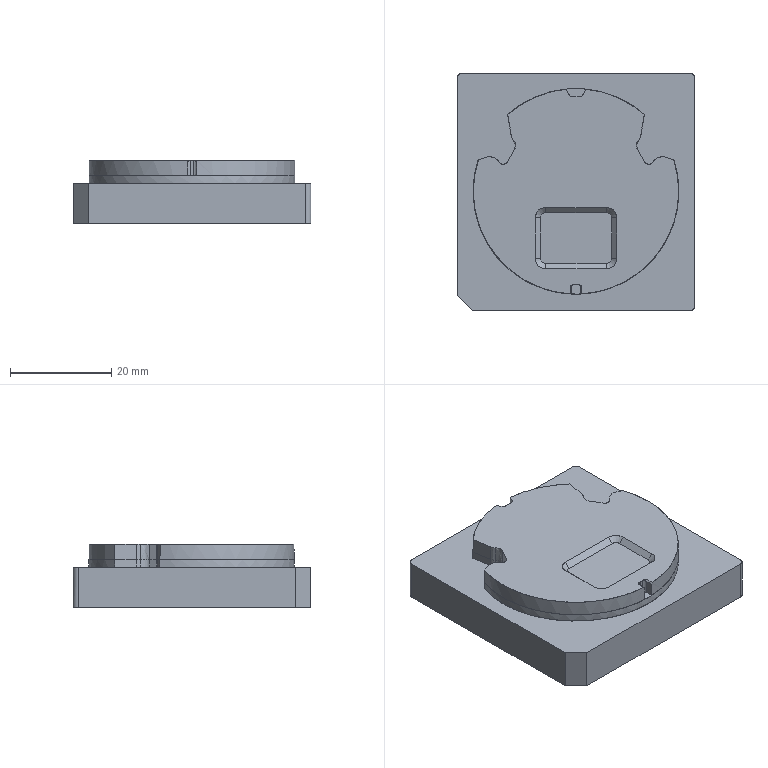NC program | PowerMill | posted with a generic post | part box 47 x 47 x 12.511 mm
Lines 3814 to 4800 of 232111:
N3911 M6
N3912 S18000 M03
N3913 G00 G90 X0.0 Y0.0
N3914 G43 Z9.8015 H15
N3915
N3916 G05 P10000 R4
N3917 X15.7379 Y13.9176
N3918 Z0.8545
N3919 G01 Z-0.3455 F3000.0
N3920 X15.7225 Y13.9292 F5000.0
N3921 G03 X15.48 Y13.8941 I-0.1037 J-0.1388
N3922 G01 X14.5606 Y12.664
N3923 X14.1805 Y10.5533
N3924 X14.048 Y10.1312
N3925 X13.8339 Y9.7091
N3926 X13.4893 Y9.2284
N3927 X13.4614 Y9.1489
N3928 X13.4808 Y9.0669
N3929 X14.3834 Y7.477
N3930 G03 X14.6063 Y7.433 I0.1304 J0.074
N3931 G01 X15.1968 Y7.8958
N3932 X15.6189 Y8.1199
N3933 X16.0411 Y8.2805
N3934 X16.4632 Y8.3842
N3935 X16.8682 Y8.4427
N3936 X17.3146
N3937 X17.7296 Y8.4111
N3938 X18.5739 Y8.1829
N3939 X19.8403 Y7.72
N3940 X20.0941 Y7.5984
N3941 X20.2624 Y7.4819
N3942 X20.5487 Y7.1763
N3943 X20.6845 Y6.9495
N3944 X20.9948 Y5.9099
N3945 X21.2205 Y5.0656
N3946 X21.5288 Y3.5136
N3947 X21.6562 Y2.5328
N3948 X21.7637 Y1.2664
N3949 X21.786 Y0.4221
N3950 X21.7476 Y-1.2664
N3951 X21.5716 Y-2.9549
N3952 X21.3505 Y-4.2213
N3953 X20.9434 Y-5.9099
N3954 X20.5366 Y-7.1763
N3955 X20.0398 Y-8.4427
N3956 X19.4181 Y-9.776
N3957 X18.7603 Y-10.9755
N3958 X17.951 Y-12.2419
N3959 X17.0083 Y-13.5083
N3960 X15.9126 Y-14.7747
N3961 X14.7747 Y-15.9019
N3962 X13.5083 Y-16.9858
N3963 X12.664 Y-17.6049
N3964 X11.8804 Y-18.1517
N3965 X10.5533 Y-18.9524
N3966 X9.2869 Y-19.5988
N3967 X7.7239 Y-20.2624
N3968 X6.4951 Y-20.6845
N3969 X5.0656 Y-21.0791
N3970 X3.7992 Y-21.3429
N3971 X2.5376 Y-21.5288
N3972 X1.2664 Y-21.6389
N3973 X0.8443 Y-21.6396
N3974 X0.4341 Y-21.5288
N3975 X0.0829 Y-21.2972
N3976 X0.0001 Y-21.2725
N3977 X-0.0827 Y-21.2975
N3978 X-0.4221 Y-21.5232
N3979 X-0.8443 Y-21.6396
N3980 X-1.2664 Y-21.6389
N3981 X-2.5375 Y-21.5288
N3982 X-3.7992 Y-21.3429
N3983 X-5.0656 Y-21.0791
N3984 X-6.4951 Y-20.6845
N3985 X-7.7269 Y-20.2624
N3986 X-8.7488 Y-19.8403
N3987 X-10.1312 Y-19.179
N3988 X-11.2043 Y-18.5739
N3989 X-12.2419 Y-17.9036
N3990 X-13.5083 Y-16.9805
N3991 X-14.6241 Y-16.0411
N3992 X-15.5066 Y-15.1968
N3993 X-15.9121 Y-14.7747
N3994 X-16.8853 Y-13.6622
N3995 X-17.9488 Y-12.2419
N3996 X-18.7581 Y-10.9755
N3997 X-19.4181 Y-9.776
N3998 X-20.0398 Y-8.4427
N3999 X-20.5365 Y-7.1763
N4000 X-20.9434 Y-5.9099
N4001 X-21.2664 Y-4.6435
N4002 X-21.5288 Y-3.2569
N4003 X-21.7173 Y-1.6885
N4004 X-21.7801 Y-0.4221
N4005 X-21.7637 Y1.2664
N4006 X-21.6562 Y2.5328
N4007 X-21.5288 Y3.5149
N4008 X-21.4005 Y4.2213
N4009 X-21.121 Y5.4877
N4010 X-20.6845 Y6.9495
N4011 X-20.5503 Y7.1763
N4012 X-20.2624 Y7.4819
N4013 X-20.0957 Y7.5984
N4014 X-19.8403 Y7.72
N4015 X-18.5739 Y8.1829
N4016 X-17.7296 Y8.4111
N4017 X-17.3075 Y8.4433
N4018 X-16.8853 Y8.4434
N4019 X-16.4632 Y8.3842
N4020 X-16.0411 Y8.2805
N4021 X-15.6189 Y8.1199
N4022 X-15.1968 Y7.8958
N4023 X-14.7747 Y7.5787
N4024 X-14.6138 Y7.4355
N4025 G03 X-14.3778 Y7.4835 I0.0999 J0.1129
N4026 G01 X-13.576 Y8.8648
N4027 X-13.4828 Y9.0677
N4028 X-13.4697 Y9.1433
N4029 X-13.4958 Y9.2156
N4030 X-13.837 Y9.7091
N4031 X-14.048 Y10.1312
N4032 X-14.1814 Y10.5533
N4033 X-14.3525 Y11.428
N4034 X-15.0027 Y15.1968
N4035 X-14.9617 Y15.6189
N4036 X-14.7907 Y16.0411
N4037 X-14.3525 Y16.5091
N4038 X-13.5083 Y17.2179
N4039 X-12.2308 Y18.1517
N4040 X-11.3976 Y18.6865
N4041 X-10.1135 Y19.4181
N4042 X-8.8648 Y20.0225
N4043 X-7.5984 Y20.5388
N4044 X-6.332 Y20.966
N4045 X-5.0656 Y21.3114
N4046 X-3.3771 Y21.6465
N4047 X-2.1107 Y21.809
N4048 X-1.6885 Y21.8011
N4049 X-1.2664 Y21.6731
N4050 X-1.0252 Y21.5288
N4051 X-0.8443 Y21.373
N4052 X-0.6349 Y21.1067
N4053 X-0.3437 Y20.503
N4054 X-0.2885 Y20.4413
N4055 X-0.2089 Y20.4182
N4056 X0.2081 Y20.4173
N4057 X0.2877 Y20.4399
N4058 X0.3431 Y20.5012
N4059 X0.6402 Y21.1067
N4060 X0.8443 Y21.373
N4061 X1.0221 Y21.5288
N4062 X1.2664 Y21.6731
N4063 X1.6885 Y21.8011
N4064 X2.1107 Y21.809
N4065 X3.3771 Y21.6465
N4066 X4.6435 Y21.406
N4067 X6.332 Y20.966
N4068 X7.5984 Y20.5388
N4069 X8.8648 Y20.0225
N4070 X10.1312 Y19.4083
N4071 X10.8809 Y18.996
N4072 X12.2419 Y18.1446
N4073 X13.3961 Y17.3075
N4074 X14.4068 Y16.4632
N4075 X14.7747 Y16.0676
N4076 X14.9617 Y15.6189
N4077 X15.0027 Y15.1968
N4078 X14.9408 Y14.7747
N4079 X14.5606 Y12.664
N4080 X15.7379 Y13.9207 Z-0.4819
N4081 X15.7225 Y13.9322
N4082 G03 X15.4801 Y13.8967 I-0.1035 J-0.139
N4083 G01 X14.5623 Y12.6637
N4084 X14.3734 Y11.6083
N4085 X14.1826 Y10.5533
N4086 X14.0498 Y10.1312
N4087 X13.8389 Y9.7091
N4088 X13.4878 Y9.2236
N4089 X13.48 Y9.2088
N4090 X13.4631 Y9.1479
N4091 X13.4733 Y9.0856
N4092 X13.4807 Y9.0669
N4093 X14.3774 Y7.4874
N4094 X14.385 Y7.4754
N4095 X14.3937 Y7.4641
N4096 G03 X14.6056 Y7.4341 I0.1201 J0.0845
N4097 G01 X15.1968 Y7.8973
N4098 X15.6189 Y8.1199
N4099 X16.0411 Y8.2822
N4100 X16.4632 Y8.3842
N4101 X16.8455 Y8.4427
N4102 X17.3146
N4103 X17.7296 Y8.412
N4104 X18.5739 Y8.1841
N4105 X19.8403 Y7.7215
N4106 X20.0981 Y7.5984
N4107 X20.2624 Y7.4845
N4108 X20.5543 Y7.1763
N4109 X20.6845 Y6.9524
N4110 X20.7592 Y6.7541
N4111 X20.946 Y6.0734
N4112 X20.9948 Y5.9099
N4113 X21.145 Y5.3481
N4114 X21.2224 Y5.0656
N4115 X21.5288 Y3.5216
N4116 X21.6562 Y2.5328
N4117 X21.7637 Y1.2664
N4118 X21.7879 Y0.4221
N4119 X21.7489 Y-1.2664
N4120 X21.5732 Y-2.9549
N4121 X21.4247 Y-3.8001
N4122 X21.2667 Y-4.6435
N4123 X20.9434 Y-5.9099
N4124 X20.5366 Y-7.1763
N4125 X20.0398 Y-8.4427
N4126 X19.4181 Y-9.776
N4127 X18.7617 Y-10.9755
N4128 X17.9511 Y-12.2419
N4129 X17.9311 Y-12.2686
N4130 X17.0083 Y-13.5082
N4131 X16.9663 Y-13.5567
N4132 X16.8853 Y-13.6649
N4133 X16.4632 Y-14.1597
N4134 X16.183 Y-14.4628
N4135 X15.9126 Y-14.7746
N4136 X15.7049 Y-14.9811
N4137 X15.5067 Y-15.1968
N4138 X14.8424 Y-15.8348
N4139 X14.7746 Y-15.9019
N4140 X14.755 Y-15.9187
N4141 X14.6276 Y-16.0411
N4142 X13.5083 Y-16.9858
N4143 X12.7021 Y-17.5773
N4144 X11.8837 Y-18.1517
N4145 X10.5533 Y-18.9538
N4146 X9.2869 Y-19.5989
N4147 X9.2363 Y-19.6203
N4148 X7.7239 Y-20.2624
N4149 X7.6482 Y-20.2883
N4150 X7.5984 Y-20.3093
N4151 X7.3606 Y-20.3872
N4152 X6.4951 Y-20.6845
N4153 X6.2004 Y-20.7664
N4154 X5.9099 Y-20.8621
N4155 X5.0656 Y-21.0791
N4156 X4.2213 Y-21.263
N4157 X4.0093 Y-21.2978
N4158 X3.7992 Y-21.3428
N4159 X2.6329 Y-21.5147
N4160 X2.5439 Y-21.5288
N4161 X1.2664 Y-21.6392
N4162 X0.8443 Y-21.6495
N4163 X0.4221 Y-21.5713
N4164 X0.3134 Y-21.5288
N4165 X0.0739 Y-21.3845
N4166 X-0.0005 Y-21.363
N4167 X-0.0756 Y-21.3814
N4168 X-0.4221 Y-21.5713
N4169 X-0.8443 Y-21.6495
N4170 X-1.2664 Y-21.6392
N4171 X-2.5419 Y-21.5288
N4172 X-3.3771 Y-21.4061
N4173 X-3.4088 Y-21.4003
N4174 X-3.7992 Y-21.3428
N4175 X-4.433 Y-21.2139
N4176 X-5.0656 Y-21.0791
N4177 X-5.4862 Y-20.9648
N4178 X-5.9099 Y-20.8621
N4179 X-6.2003 Y-20.7661
N4180 X-6.4951 Y-20.6845
N4181 X-7.6618 Y-20.2847
N4182 X-7.7372 Y-20.2595
N4183 X-7.8101 Y-20.228
N4184 X-8.7488 Y-19.8402
N4185 X-9.0152 Y-19.7136
N4186 X-9.2869 Y-19.5986
N4187 X-9.8824 Y-19.3
N4188 X-10.475 Y-18.996
N4189 X-10.837 Y-18.7802
N4190 X-11.2043 Y-18.5738
N4191 X-11.5416 Y-18.3569
N4192 X-11.8861 Y-18.1517
N4193 X-12.5052 Y-17.7296
N4194 X-13.5083 Y-16.983
N4195 X-14.6273 Y-16.0411
N4196 X-14.7473 Y-15.9231
N4197 X-15.5066 Y-15.1968
N4198 X-15.8535 Y-14.8357
N4199 X-15.9155 Y-14.7747
N4200 X-16.8853 Y-13.6649
N4201 X-17.9508 Y-12.2419
N4202 X-18.76 Y-10.9755
N4203 X-18.9495 Y-10.641
N4204 X-19.1291 Y-10.3012
N4205 X-19.4181 Y-9.776
N4206 X-19.5335 Y-9.5287
N4207 X-19.6602 Y-9.2869
N4208 X-19.9644 Y-8.6022
N4209 X-20.2624 Y-7.9147
N4210 X-20.3927 Y-7.543
N4211 X-20.5365 Y-7.1763
N4212 X-20.7435 Y-6.5442
N4213 X-20.9433 Y-5.9099
N4214 X-21.2004 Y-4.9021
N4215 X-21.2697 Y-4.6435
N4216 X-21.5288 Y-3.2633
N4217 X-21.7179 Y-1.6885
N4218 X-21.721 Y-1.6137
N4219 X-21.78 Y-0.4221
N4220 X-21.7785 Y-0.211
N4221 X-21.7877 Y0.0
N4222 X-21.7637 Y1.2664
N4223 X-21.6562 Y2.5328
N4224 X-21.6555 Y2.5376
N4225 X-21.5288 Y3.5149
N4226 X-21.4005 Y4.2213
N4227 X-21.1231 Y5.478
N4228 X-21.121 Y5.4877
N4229 X-20.7601 Y6.7541
N4230 X-20.6845 Y6.9524
N4231 X-20.553 Y7.1763
N4232 X-20.2624 Y7.4845
N4233 X-20.1003 Y7.5984
N4234 X-19.8403 Y7.7215
N4235 X-18.5739 Y8.1841
N4236 X-17.7296 Y8.412
N4237 X-17.3075 Y8.4438
N4238 X-17.0998 Y8.4433
N4239 X-16.8853 Y8.4434
N4240 X-16.8786 Y8.4429
N4241 X-16.8719 Y8.4427
N4242 X-16.8464
N4243 X-16.4632 Y8.3842
N4244 X-16.0411 Y8.2822
N4245 X-15.6189 Y8.1199
N4246 X-15.1968 Y7.8973
N4247 X-14.7747 Y7.5788
N4248 X-14.614 Y7.4367
N4249 G03 X-14.3848 Y7.4738 I0.0994 J0.1123
N4250 G01 X-13.5788 Y8.8648
N4251 X-13.4847 Y9.0685
N4252 X-13.4714 Y9.1446
N4253 X-13.4977 Y9.2171
N4254 X-13.84 Y9.7091
N4255 X-14.0498 Y10.1312
N4256 X-14.1844 Y10.5533
N4257 X-14.2133 Y10.7167
N4258 X-14.3525 Y11.428
N4259 X-14.6757 Y13.3132
N4260 X-15.0077 Y15.1968
N4261 X-14.964 Y15.6189
N4262 X-14.7924 Y16.0411
N4263 X-14.4139 Y16.4632
N4264 X-13.748 Y17.0166
N4265 X-13.5082 Y17.2179
N4266 X-13.4877 Y17.2329
N4267 X-13.398 Y17.3075
N4268 X-12.2328 Y18.1517
N4269 X-11.563 Y18.5791
N4270 X-10.8867 Y18.996
N4271 X-10.1135 Y19.4181
N4272 X-9.267 Y19.8403
N4273 X-8.9335 Y19.9892
N4274 X-8.5971 Y20.1316
N4275 X-8.0205 Y20.3823
N4276 X-7.8077 Y20.4559
N4277 X-7.5984 Y20.5388
N4278 X-6.9672 Y20.7585
N4279 X-6.332 Y20.966
N4280 X-5.6978 Y21.1375
N4281 X-5.0656 Y21.3161
N4282 X-3.7992 Y21.573
N4283 X-3.5871 Y21.6037
N4284 X-3.3771 Y21.6464
N4285 X-2.2152 Y21.7955
N4286 X-2.1107 Y21.8102
N4287 X-1.6885 Y21.8062
N4288 X-1.2664 Y21.6747
N4289 X-1.0211 Y21.5288
N4290 X-0.8443 Y21.3752
N4291 X-0.6347 Y21.1067
N4292 X-0.3437 Y20.5031
N4293 X-0.2885 Y20.4413
N4294 X-0.2089 Y20.4182
N4295 X0.2079 Y20.4173
N4296 X0.2876 Y20.44
N4297 X0.343 Y20.5015
N4298 X0.638 Y21.1067
N4299 X0.8443 Y21.3752
N4300 X1.0211 Y21.5288
N4301 X1.2664 Y21.6747
N4302 X1.6885 Y21.8062
N4303 X2.1107 Y21.8102
N4304 X3.3771 Y21.647
N4305 X4.2224 Y21.4872
N4306 X5.0656 Y21.316
N4307 X6.332 Y20.9672
N4308 X7.5984 Y20.5389
N4309 X8.8648 Y20.0225
N4310 X10.1312 Y19.4083
N4311 X10.8852 Y18.996
N4312 X12.2419 Y18.1453
N4313 X13.398 Y17.3075
N4314 X14.4107 Y16.4632
N4315 X14.7747 Y16.0701
N4316 X14.964 Y15.6189
N4317 X15.0077 Y15.1968
N4318 X14.7864 Y13.93
N4319 X14.5623 Y12.6637
N4320 X15.7373 Y13.9068 Z-0.6184
N4321 X15.7219 Y13.9183
N4322 G03 X15.4795 Y13.8825 I-0.1033 J-0.1391
N4323 G01 X14.5731 Y12.6618
N4324 X14.2749 Y10.9755
N4325 X14.1847 Y10.5533
N4326 X14.0515 Y10.1312
N4327 X13.8424 Y9.7091
N4328 X13.4916 Y9.2261
N4329 X13.4632 Y9.1462
N4330 X13.4826 Y9.0637
N4331 X14.3838 Y7.4804
N4332 G03 X14.6067 Y7.4366 I0.1304 J0.0743
N4333 G01 X15.1968 Y7.8988
N4334 X15.6189 Y8.1199
N4335 X16.0411 Y8.2839
N4336 X16.4632 Y8.3842
N4337 X16.4722 Y8.3855
N4338 X16.8455 Y8.4426
N4339 X16.9067 Y8.4465
N4340 X16.9679 Y8.4426
N4341 X17.3146
N4342 X17.6939 Y8.4146
N4343 X17.7296 Y8.4132
N4344 X18.5739 Y8.1854
N4345 X19.8403 Y7.723
N4346 X20.1021 Y7.5984
N4347 X20.2624 Y7.4871
N4348 X20.5559 Y7.1763
N4349 X20.6845 Y6.9553
N4350 X20.7625 Y6.7541
N4351 X20.9795 Y5.9611
N4352 X20.9947 Y5.9098
N4353 X21.0497 Y5.7043
N4354 X21.2244 Y5.0656
N4355 X21.5288 Y3.5296
N4356 X21.6562 Y2.5328
N4357 X21.7351 Y1.6885
N4358 X21.7688 Y1.1211
N4359 X21.7841 Y0.553
N4360 X21.7897 Y0.4221
N4361 X21.7498 Y-1.2664
N4362 X21.5747 Y-2.9549
N4363 X21.4862 Y-3.4437
N4364 X21.3504 Y-4.2213
N4365 X21.3299 Y-4.3064
N4366 X21.2688 Y-4.6435
N4367 X21.2147 Y-4.8471
N4368 X20.9433 Y-5.9099
N4369 X20.8763 Y-6.1194
N4370 X20.8201 Y-6.332
N4371 X20.6726 Y-6.7522
N4372 X20.5366 Y-7.1763
N4373 X20.3928 Y-7.5449
N4374 X20.2624 Y-7.9184
N4375 X20.0398 Y-8.4427
N4376 X19.4181 Y-9.776
N4377 X18.7631 Y-10.9755
N4378 X17.9521 Y-12.2419
N4379 X17.7109 Y-12.5643
N4380 X17.0082 Y-13.5082
N4381 X16.981 Y-13.5397
N4382 X16.8853 Y-13.6675
N4383 X16.4632 Y-14.1597
N4384 X16.183 Y-14.4628
N4385 X15.9126 Y-14.7746
N4386 X15.7049 Y-14.9811
N4387 X15.5067 Y-15.1968
N4388 X14.7959 Y-15.8808
N4389 X14.7746 Y-15.9019
N4390 X14.7689 Y-15.9067
N4391 X14.6293 Y-16.0411
N4392 X13.5083 Y-16.9859
N4393 X13.0699 Y-17.3188
N4394 X12.6198 Y-17.6356
N4395 X11.8871 Y-18.1517
N4396 X10.5533 Y-18.9552
N4397 X9.2869 Y-19.5991
N4398 X9.1754 Y-19.646
N4399 X7.7239 Y-20.2623
N4400 X7.5153 Y-20.3383
N4401 X7.3041 Y-20.4065
N4402 X6.4951 Y-20.6844
N4403 X6.2003 Y-20.7671
N4404 X5.9099 Y-20.8636
N4405 X5.8219 Y-20.8846
N4406 X5.0656 Y-21.0791
N4407 X4.4008 Y-21.2239
N4408 X4.196 Y-21.2717
N4409 X3.9882 Y-21.3034
N4410 X3.7992 Y-21.3428
N4411 X2.8483 Y-21.4829
N4412 X2.5569 Y-21.5288
N4413 X1.6885 Y-21.6067
N4414 X1.2668 Y-21.6366
N4415 X0.8443 Y-21.6526
N4416 X0.4221 Y-21.5733
N4417 X0.3093 Y-21.5288
N4418 X0.0738 Y-21.3869
N4419 X-0.0005 Y-21.3654
N4420 X-0.0756 Y-21.3837
N4421 X-0.4221 Y-21.5733
N4422 X-0.8443 Y-21.6526
N4423 X-1.2664 Y-21.6394
N4424 X-2.5328 Y-21.5311
N4425 X-3.3782 Y-21.4062
N4426 X-4.2213 Y-21.2668
N4427 X-4.4312 Y-21.215
N4428 X-4.6435 Y-21.1744
N4429 X-5.1754 Y-21.0474
N4430 X-5.7053 Y-20.9125
N4431 X-5.9099 Y-20.8636
N4432 X-6.2003 Y-20.7668
N4433 X-6.4951 Y-20.6844
N4434 X-7.5967 Y-20.3069
N4435 X-7.7316 Y-20.2624
N4436 X-8.7517 Y-19.8403
N4437 X-9.0166 Y-19.7135
N4438 X-9.2869 Y-19.5985
N4439 X-9.8824 Y-19.3
N4440 X-10.475 Y-18.996
N4441 X-11.1839 Y-18.5794
N4442 X-11.8861 Y-18.1517
N4443 X-12.1587 Y-17.9658
N4444 X-12.2419 Y-17.9128
N4445 X-12.8791 Y-17.4547
N4446 X-13.5083 Y-16.9855
N4447 X-14.6305 Y-16.0411
N4448 X-14.8547 Y-15.8203
N4449 X-15.5065 Y-15.1967
N4450 X-15.8293 Y-14.8608
N4451 X-15.9167 Y-14.7747
N4452 X-16.8853 Y-13.6675
N4453 X-17.9529 Y-12.2419
N4454 X-18.7619 Y-10.9755
N4455 X-18.9632 Y-10.6179
N4456 X-19.1545 Y-10.2548
N4457 X-19.418 Y-9.776
N4458 X-19.5342 Y-9.5286
N4459 X-19.6617 Y-9.2869
N4460 X-19.8459 Y-8.8626
N4461 X-20.0397 Y-8.4426
N4462 X-20.1458 Y-8.1783
N4463 X-20.2624 Y-7.9185
N4464 X-20.3928 Y-7.5449
N4465 X-20.5364 Y-7.1762
N4466 X-20.6727 Y-6.7522
N4467 X-20.8205 Y-6.332
N4468 X-21.0512 Y-5.4892
N4469 X-21.271 Y-4.6435
N4470 X-21.5288 Y-3.2697
N4471 X-21.7185 Y-1.6885
N4472 X-21.7807 Y-0.4221
N4473 X-21.7801 Y0.4222
N4474 X-21.7637 Y1.2664
N4475 X-21.7135 Y1.9023
N4476 X-21.6555 Y2.5376
N4477 X-21.558 Y3.289
N4478 X-21.5348 Y3.4926
N4479 X-21.4962 Y3.694
N4480 X-21.3215 Y4.5935
N4481 X-21.121 Y5.4877
N4482 X-20.8185 Y6.5492
N4483 X-20.7621 Y6.7557
N4484 X-20.6845 Y6.9553
N4485 X-20.5558 Y7.1763
N4486 X-20.2624 Y7.4871
N4487 X-20.1028 Y7.5984
N4488 X-19.8403 Y7.723
N4489 X-18.5739 Y8.1854
N4490 X-17.7296 Y8.4132
N4491 X-17.3075 Y8.4443
N4492 X-17.0029 Y8.4433
N4493 X-16.8857 Y8.4443
N4494 X-16.7693 Y8.4308
N4495 X-16.4632 Y8.3841
N4496 X-16.0857 Y8.2929
N4497 X-16.0411 Y8.2839
N4498 X-15.6189 Y8.1199
N4499 X-15.1968 Y7.8988
N4500 X-14.7747 Y7.5792
N4501 X-14.6152 Y7.439
N4502 G03 X-14.3863 Y7.4764 I0.0991 J0.1126
N4503 G01 X-13.5816 Y8.8648
N4504 X-13.4867 Y9.0677
N4505 X-13.4731 Y9.144
N4506 X-13.4995 Y9.217
N4507 X-13.8424 Y9.7091
N4508 X-14.0515 Y10.1312
N4509 X-14.1861 Y10.5533
N4510 X-14.2973 Y11.1461
N4511 X-14.3524 Y11.428
N4512 X-14.3789 Y11.5815
N4513 X-14.4236 Y11.8197
N4514 X-14.9466 Y14.7747
N4515 X-15.009 Y15.1968
N4516 X-14.9663 Y15.6189
N4517 X-14.7941 Y16.0411
N4518 X-14.4158 Y16.4632
N4519 X-13.5604 Y17.174
N4520 X-13.5082 Y17.2179
N4521 X-13.5037 Y17.2211
N4522 X-13.3998 Y17.3075
N4523 X-12.2348 Y18.1517
N4524 X-11.8197 Y18.4228
N4525 X-11.5161 Y18.6108
N4526 X-11.2092 Y18.7937
N4527 X-10.8867 Y18.996
N4528 X-10.1564 Y19.3933
N4529 X-9.4137 Y19.7671
N4530 X-9.2712 Y19.8403
N4531 X-9.0661 Y19.9272
N4532 X-8.8648 Y20.0224
N4533 X-8.6687 Y20.1023
N4534 X-8.0205 Y20.3842
N4535 X-7.6737 Y20.508
N4536 X-7.5404 Y20.5603
N4537 X-7.4041 Y20.6043
N4538 X-6.7541 Y20.8363
N4539 X-5.911 Y21.0811
N4540 X-5.0656 Y21.318
N4541 X-3.7992 Y21.5744
N4542 X-3.5871 Y21.6044
N4543 X-3.3771 Y21.6464
N4544 X-2.3222 Y21.7817
N4545 X-2.1107 Y21.8114
N4546 X-1.6885 Y21.8073
N4547 X-1.2664 Y21.6764
N4548 X-1.0201 Y21.5288
N4549 X-0.8443 Y21.3758
N4550 X-0.6345 Y21.1067
N4551 X-0.3437 Y20.5031
N4552 X-0.2885 Y20.4413
N4553 X-0.2089 Y20.4182
N4554 X0.2076 Y20.4173
N4555 X0.2875 Y20.4401
N4556 X0.3429 Y20.5019
N4557 X0.6358 Y21.1067
N4558 X0.8443 Y21.3758
N4559 X1.02 Y21.5288
N4560 X1.2664 Y21.6764
N4561 X1.6885 Y21.8073
N4562 X2.1107 Y21.8114
N4563 X3.3771 Y21.6476
N4564 X4.0556 Y21.5188
N4565 X4.7328 Y21.3829
N4566 X5.0656 Y21.3179
N4567 X6.332 Y20.9684
N4568 X7.1784 Y20.6825
N4569 X8.0205 Y20.3842
N4570 X8.6676 Y20.1028
N4571 X9.1947 Y19.8742
N4572 X9.7069 Y19.6141
N4573 X10.1312 Y19.4083
N4574 X10.7898 Y19.0481
N4575 X10.8895 Y18.996
N4576 X12.2419 Y18.1467
N4577 X13.3999 Y17.3075
N4578 X14.4146 Y16.4632
N4579 X14.7747 Y16.0725
N4580 X14.9663 Y15.6189
N4581 X15.009 Y15.1968
N4582 X14.9468 Y14.7747
N4583 X14.5731 Y12.6618
N4584 X15.7368 Y13.9039 Z-0.7548
N4585 X15.7213 Y13.9154
N4586 G03 X15.479 Y13.8796 I-0.1032 J-0.1391
N4587 G01 X14.5744 Y12.6616
N4588 X14.2761 Y10.9755
N4589 X14.1869 Y10.5533
N4590 X14.0533 Y10.1312
N4591 X13.8438 Y9.7091
N4592 X13.4948 Y9.2294
N4593 X13.4664 Y9.1496
N4594 X13.4856 Y9.0672
N4595 X14.3842 Y7.4827
N4596 G03 X14.6072 Y7.4386 I0.1305 J0.074
N4597 G01 X15.1968 Y7.9003
N4598 X15.6189 Y8.1199
N4599 X16.0411 Y8.2854
N4600 X16.0851 Y8.2944
N4601 X16.4632 Y8.3841
N4602 X16.6737 Y8.419
N4603 X16.8853 Y8.4458
N4604 X16.9653 Y8.4427
N4605 X17.4027
N4606 X17.7296 Y8.4144
N4607 X18.5739 Y8.1867
N4608 X19.8403 Y7.7245
N4609 X20.1053 Y7.5984
N4610 X20.2624 Y7.4893
N4611 X20.5575 Y7.1763
N4612 X20.6845 Y6.9581
N4613 X20.7639 Y6.7541
N4614 X21.2263 Y5.0656
N4615 X21.5288 Y3.5376
N4616 X21.5367 Y3.4675
N4617 X21.6562 Y2.5328
N4618 X21.7173 Y1.9002
N4619 X21.7636 Y1.2664
N4620 X21.7812 Y0.6517
N4621 X21.791 Y0.4221
N4622 X21.7507 Y-1.2664
N4623 X21.5763 Y-2.9549
N4624 X21.4473 Y-3.6662
N4625 X21.3503 Y-4.2213
N4626 X21.3352 Y-4.2841
N4627 X21.27 Y-4.6435
N4628 X21.0512 Y-5.489
N4629 X20.8229 Y-6.332
N4630 X20.6738 Y-6.7521
N4631 X20.5365 Y-7.1762
N4632 X20.393 Y-7.5465
N4633 X20.2624 Y-7.9216
N4634 X20.0398 Y-8.4427
N4635 X19.4181 Y-9.7761
N4636 X18.7645 Y-10.9755
N4637 X17.9535 Y-12.2419
N4638 X17.3952 Y-12.9882
N4639 X17.0082 Y-13.5082
N4640 X16.9106 Y-13.6383
N4641 X16.8046 Y-13.7616
N4642 X16.4632 Y-14.1597
N4643 X16.1844 Y-14.464
N4644 X15.9127 Y-14.7747
N4645 X15.7053 Y-14.9814
N4646 X15.5067 Y-15.1968
N4647 X14.7959 Y-15.8807
N4648 X14.7746 Y-15.9018
N4649 X14.7689 Y-15.9067
N4650 X14.6975 Y-15.9754
N4651 X14.631 Y-16.0411
N4652 X13.5083 Y-16.9859
N4653 X13.0861 Y-17.3087
N4654 X11.8904 Y-18.1517
N4655 X10.5533 Y-18.9565
N4656 X9.2869 Y-19.5992
N4657 X8.4439 Y-19.9582
N4658 X7.5984 Y-20.3113
N4659 X6.7559 Y-20.5935
N4660 X5.9099 Y-20.8652
N4661 X5.0677 Y-21.0756
N4662 X4.2213 Y-21.2683
N4663 X3.3961 Y-21.4022
N4664 X2.5698 Y-21.5288
N4665 X1.6885 Y-21.6079
N4666 X1.2666 Y-21.6357
N4667 X0.8443 Y-21.6556
N4668 X0.4221 Y-21.5752
N4669 X0.3053 Y-21.5288
N4670 X0.0775 Y-21.3914
N4671 X0.0 Y-21.3699
N4672 X-0.0775 Y-21.3914
N4673 X-0.3052 Y-21.5288
N4674 X-0.4221 Y-21.5752
N4675 X-0.8443 Y-21.6556
N4676 X-1.2664 Y-21.6397
N4677 X-2.5705 Y-21.5288
N4678 X-3.3965 Y-21.4026
N4679 X-4.2213 Y-21.2684
N4680 X-4.4311 Y-21.2157
N4681 X-4.6434 Y-21.1744
N4682 X-5.0732 Y-21.0735
N4683 X-5.5006 Y-20.9629
N4684 X-5.9099 Y-20.8652
N4685 X-6.2864 Y-20.742
N4686 X-6.4951 Y-20.6844
N4687 X-7.0454 Y-20.4947
N4688 X-7.5984 Y-20.3127
N4689 X-7.6688 Y-20.2831
N4690 X-7.7316 Y-20.2624
N4691 X-8.7517 Y-19.8402
N4692 X-9.0164 Y-19.7146
N4693 X-9.2869 Y-19.6021
N4694 X-10.1312 Y-19.1791
N4695 G02 X-12.5052 Y-17.7295 I11.2235 J21.0501
N4696 G01 X-13.1229 Y-17.2697
N4697 X-13.5083 Y-16.988
N4698 X-14.6322 Y-16.0411
N4699 X-14.9154 Y-15.7622
N4700 X-15.5065 Y-15.1967
N4701 X-15.8058 Y-14.8851
N4702 X-15.918 Y-14.7747
N4703 X-16.8853 Y-13.6699
N4704 X-17.9549 Y-12.2419
N4705 X-18.7637 Y-10.9755
N4706 X-18.9629 Y-10.6172
N4707 X-19.1545 Y-10.2548
N4708 X-19.418 Y-9.7759
N4709 X-19.535 Y-9.5287
N4710 X-19.6631 Y-9.2869
N4711 X-19.8466 Y-8.8627
N4712 X-20.0396 Y-8.4426
N4713 X-20.0882 Y-8.3187
N4714 X-20.2624 Y-7.9221
N4715 X-20.3929 Y-7.5468
N4716 X-20.5364 Y-7.1762
N4717 X-20.6738 Y-6.7521
N4718 X-20.8231 Y-6.332
N4719 X-21.0508 Y-5.4886
N4720 X-21.2721 Y-4.6435
N4721 X-21.5288 Y-3.2761
N4722 X-21.719 Y-1.6885
N4723 X-21.7619 Y-0.8446
N4724 X-21.7913 Y0.0
N4725 X-21.7823 Y0.2791
N4726 G02 X-21.6554 Y2.5376 I20.0409 J0.0069
N4727 G01 X-21.558 Y3.289
N4728 X-21.5269 Y3.5411
N4729 X-21.4786 Y3.7906
N4730 X-21.3555 Y4.4288
N4731 X-21.2253 Y5.0656
N4732 X-21.1678 Y5.2754
N4733 X-21.1209 Y5.4877
N4734 X-20.8546 Y6.4222
N4735 X-20.7639 Y6.7541
N4736 X-20.6845 Y6.9581
N4737 X-20.5575 Y7.1763
N4738 X-20.2624 Y7.4893
N4739 X-20.1053 Y7.5984
N4740 X-19.8403 Y7.7245
N4741 X-18.5739 Y8.1867
N4742 X-17.7296 Y8.4144
N4743 X-17.4027 Y8.4427
N4744 X-17.3296
N4745 X-17.3075 Y8.4443
N4746 X-17.0029 Y8.4432
N4747 X-16.8853 Y8.4433
N4748 X-16.8795 Y8.4429
N4749 X-16.8737 Y8.4428
N4750 X-16.7924 Y8.4402
N4751 X-16.7131 Y8.4222
N4752 X-16.4632 Y8.3841
N4753 X-16.1271 Y8.3029
N4754 X-16.0411 Y8.2854
N4755 X-15.6189 Y8.1199
N4756 X-15.1968 Y7.9003
N4757 X-14.7747 Y7.5807
N4758 X-14.6152 Y7.4407
N4759 G03 X-14.3864 Y7.4783 I0.099 J0.1127
N4760 G01 X-13.5844 Y8.8648
N4761 X-13.4886 Y9.0671
N4762 X-13.4748 Y9.1438
N4763 X-13.5011 Y9.217
N4764 X-13.8438 Y9.7091
N4765 X-14.0533 Y10.1312
N4766 X-14.1874 Y10.5533
N4767 X-14.2761 Y10.9755
N4768 X-14.9483 Y14.7747
N4769 X-15.0102 Y15.1968
N4770 X-14.9686 Y15.6189
N4771 X-14.7958 Y16.0411
N4772 X-14.4176 Y16.4632
N4773 X-13.4017 Y17.3075
N4774 X-12.2369 Y18.1517
N4775 X-11.9444 Y18.3438
N4776 X-11.6462 Y18.5268
N4777 X-10.8902 Y18.9903
N4778 X-10.1135 Y19.418
N4779 X-9.4405 Y19.7536
N4780 X-9.2746 Y19.8403
N4781 X-8.9397 Y19.9861
N4782 X-8.8375 Y20.0345
N4783 X-8.7324 Y20.0763
N4784 X-8.0205 Y20.3862
N4785 X-7.6378 Y20.5226
N4786 X-7.5983 Y20.5387
N4787 X-7.4928 Y20.5743
N4788 X-6.7541 Y20.8376
N4789 X-5.9107 Y21.0813
N4790 X-5.0656 Y21.3192
N4791 X-3.7992 Y21.5758
N4792 X-2.956 Y21.7017
N4793 X-2.1107 Y21.8126
N4794 X-1.6885 Y21.8084
N4795 X-1.2664 Y21.678
N4796 X-1.0191 Y21.5288
N4797 X-0.8443 Y21.3764
N4798 X-0.6342 Y21.1067
N4799 X-0.3437 Y20.5031
N4800 X-0.2885 Y20.4413
N4801 X-0.2089 Y20.4182
N4802 X0.2074 Y20.4173
N4803 X0.2874 Y20.4402
N4804 X0.3428 Y20.5022
N4805 X0.6341 Y21.1067
N4806 X0.8443 Y21.3764
N4807 X1.019 Y21.5288
N4808 X1.2664 Y21.678
N4809 X1.6885 Y21.8084
N4810 X2.1107 Y21.8126
N4811 X3.3771 Y21.6482
N4812 X3.7567 Y21.5742
N4813 X4.6434 Y21.4058
N4814 X4.7108 Y21.3883
N4815 X5.0656 Y21.3192
N4816 X6.332 Y20.9697
N4817 X7.1774 Y20.6812
N4818 X8.0205 Y20.3862
N4819 X8.7274 Y20.0784
N4820 X8.8359 Y20.0353
N4821 X8.9414 Y19.9852
N4822 X9.2869 Y19.8348
N4823 X9.7059 Y19.6152
N4824 X10.1312 Y19.4082
N4825 X10.7294 Y19.0811
N4826 X10.8922 Y18.996
N4827 X12.2419 Y18.1482
N4828 X13.4017 Y17.3075
N4829 X14.4176 Y16.4632
N4830 X14.7747 Y16.075
N4831 X14.9686 Y15.6189
N4832 X15.0102 Y15.1968
N4833 X14.9483 Y14.7747
N4834 X14.5744 Y12.6616
N4835 X15.7363 Y13.9015 Z-0.8913
N4836 X15.7209 Y13.913
N4837 G03 X15.4785 Y13.8772 I-0.1033 J-0.1391
N4838 G01 X14.5756 Y12.6614
N4839 X14.2773 Y10.9755
N4840 X14.1886 Y10.5533
N4841 X14.0551 Y10.1312
N4842 X13.8451 Y9.7091
N4843 X13.5003 Y9.2246
N4844 X13.473 Y9.1434
N4845 X13.49 Y9.0595
N4846 X14.3842 Y7.4827
N4847 G03 X14.6071 Y7.4389 I0.1303 J0.074
N4848 G01 X15.1968 Y7.9017
N4849 X15.6189 Y8.12
N4850 X16.0411 Y8.2866
N4851 X16.1282 Y8.3045
N4852 X16.4632 Y8.3841
N4853 X16.6323 Y8.4091
N4854 X16.7999 Y8.4427
N4855 X16.8645
N4856 X16.9143 Y8.4472
N4857 X16.964 Y8.4427
N4858 X17.4854
N4859 X17.7296 Y8.4156
N4860 X18.5739 Y8.1879
N4861 X19.8403 Y7.7259
N4862 X20.1078 Y7.5984
N4863 X20.2624 Y7.4909
N4864 X20.5591 Y7.1763
N4865 X20.6845 Y6.961
N4866 X20.7651 Y6.7541
N4867 X21.2281 Y5.0656
N4868 X21.5288 Y3.5456
N4869 X21.5448 Y3.4039
N4870 X21.6561 Y2.5328
N4871 X21.7201 Y1.848
N4872 X21.7605 Y1.2942
N4873 X21.7786 Y0.7393
N4874 X21.7922 Y0.4221
N4875 X21.7517 Y-1.2664
N4876 X21.5778 Y-2.9549
N4877 X21.4106 Y-3.8759
N4878 X21.3503 Y-4.2213
N4879 X21.3405 Y-4.2616
N4880 X21.2712 Y-4.6435
N4881 X21.0508 Y-5.4886
N4882 X20.8241 Y-6.332
N4883 X20.5469 Y-7.1297
N4884 X20.2624 Y-7.9248
N4885 X20.1022 Y-8.3001
N4886 X19.9331 Y-8.6715
N4887 X19.6617 Y-9.2869
N4888 X19.5336 Y-9.5284
N4889 X19.4181 Y-9.776
N4890 X18.8198 Y-10.874
N4891 X18.766 Y-10.9755
N4892 X17.955 Y-12.2419
N4893 X17.0976 Y-13.388
N4894 X16.9269 Y-13.6161
N4895 X16.7428 Y-13.8335
N4896 X16.5235 Y-14.0918
N4897 X16.2949 Y-14.342